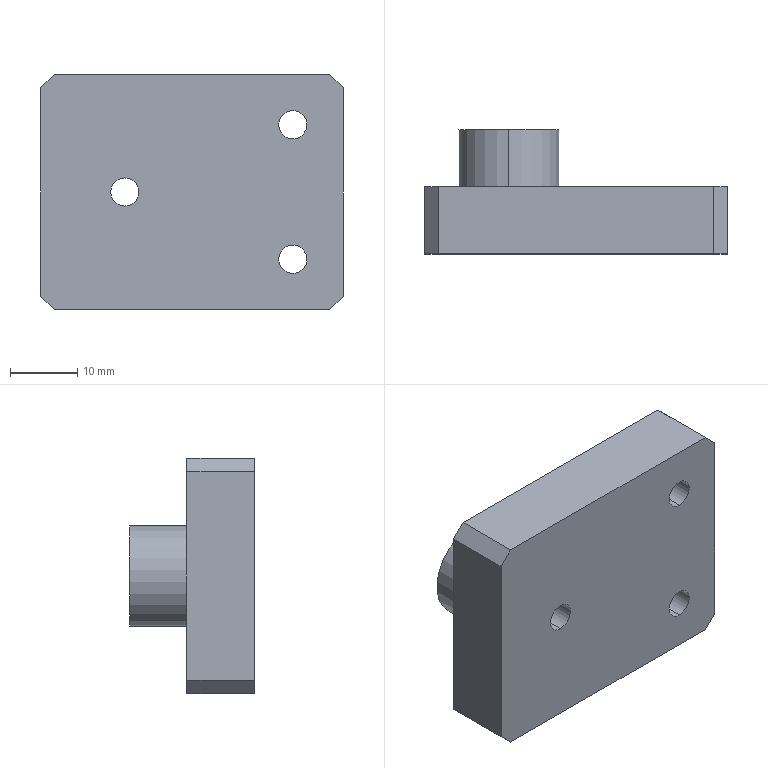Part | SolidWorks | features HoleWzd 2, ICE 2, Chamfer 1, Extrusion 1 | 1 solid | 19 faces | box 45 x 18.5 x 35 mm | volume 16639 mm3 | plane 11 | cylinder 8 | commonest cylinder face diameters 4.2 x6 15 x2
STEP:
#1=CARTESIAN_POINT('',(-10.,-5.,-2.1));
#2=VERTEX_POINT('',#1);
#3=CARTESIAN_POINT('',(-10.,-5.,2.1));
#4=VERTEX_POINT('',#3);
#5=CARTESIAN_POINT('',(-10.,-5.,0.));
#6=DIRECTION('',(0.,1.,0.));
#7=DIRECTION('',(0.,0.,1.));
#8=AXIS2_PLACEMENT_3D('',#5,#6,#7);
#9=CIRCLE('',#8,2.1);
#10=EDGE_CURVE('',#2,#4,#9,.T.);
#11=ORIENTED_EDGE('',*,*,#10,.F.);
#12=CARTESIAN_POINT('',(-10.,13.5,-2.1));
#13=VERTEX_POINT('',#12);
#14=CARTESIAN_POINT('',(-10.,13.5,-2.1));
#15=DIRECTION('',(0.,1.,0.));
#16=VECTOR('',#15,1000.);
#17=LINE('',#14,#16);
#18=EDGE_CURVE('',#2,#13,#17,.T.);
#19=ORIENTED_EDGE('',*,*,#18,.T.);
#20=CARTESIAN_POINT('',(-10.,13.5,2.1));
#21=VERTEX_POINT('',#20);
#22=CARTESIAN_POINT('',(-10.,13.5,0.));
#23=DIRECTION('',(0.,1.,0.));
#24=DIRECTION('',(0.,0.,1.));
#25=AXIS2_PLACEMENT_3D('',#22,#23,#24);
#26=CIRCLE('',#25,2.1);
#27=EDGE_CURVE('',#13,#21,#26,.T.);
#28=ORIENTED_EDGE('',*,*,#27,.T.);
#29=CARTESIAN_POINT('',(-10.,13.5,2.1));
#30=DIRECTION('',(0.,1.,0.));
#31=VECTOR('',#30,1000.);
#32=LINE('',#29,#31);
#33=EDGE_CURVE('',#4,#21,#32,.T.);
#34=ORIENTED_EDGE('',*,*,#33,.F.);
#35=EDGE_LOOP('',(#11,#19,#28,#34));
#36=FACE_OUTER_BOUND('',#35,.T.);
#37=CARTESIAN_POINT('',(-10.,13.5,0.));
#38=DIRECTION('',(0.,1.,0.));
#39=DIRECTION('',(0.,0.,1.));
#40=AXIS2_PLACEMENT_3D('',#37,#38,#39);
#41=CYLINDRICAL_SURFACE('',#40,2.1);
#42=ADVANCED_FACE('',(#36),#41,.F.);
#43=CARTESIAN_POINT('',(15.,-5.,7.9));
#44=VERTEX_POINT('',#43);
#45=CARTESIAN_POINT('',(15.,-5.,12.1));
#46=VERTEX_POINT('',#45);
#47=CARTESIAN_POINT('',(15.,-5.,10.));
#48=DIRECTION('',(0.,1.,0.));
#49=DIRECTION('',(0.,0.,1.));
#50=AXIS2_PLACEMENT_3D('',#47,#48,#49);
#51=CIRCLE('',#50,2.1);
#52=EDGE_CURVE('',#44,#46,#51,.T.);
#53=ORIENTED_EDGE('',*,*,#52,.F.);
#54=CARTESIAN_POINT('',(15.,5.,7.9));
#55=VERTEX_POINT('',#54);
#56=CARTESIAN_POINT('',(15.,5.,7.9));
#57=DIRECTION('',(0.,1.,0.));
#58=VECTOR('',#57,1000.);
#59=LINE('',#56,#58);
#60=EDGE_CURVE('',#44,#55,#59,.T.);
#61=ORIENTED_EDGE('',*,*,#60,.T.);
#62=CARTESIAN_POINT('',(15.,5.,12.1));
#63=VERTEX_POINT('',#62);
#64=CARTESIAN_POINT('',(15.,5.,10.));
#65=DIRECTION('',(0.,1.,0.));
#66=DIRECTION('',(0.,0.,1.));
#67=AXIS2_PLACEMENT_3D('',#64,#65,#66);
#68=CIRCLE('',#67,2.1);
#69=EDGE_CURVE('',#55,#63,#68,.T.);
#70=ORIENTED_EDGE('',*,*,#69,.T.);
#71=CARTESIAN_POINT('',(15.,5.,12.1));
#72=DIRECTION('',(0.,1.,0.));
#73=VECTOR('',#72,1000.);
#74=LINE('',#71,#73);
#75=EDGE_CURVE('',#46,#63,#74,.T.);
#76=ORIENTED_EDGE('',*,*,#75,.F.);
#77=EDGE_LOOP('',(#53,#61,#70,#76));
#78=FACE_OUTER_BOUND('',#77,.T.);
#79=CARTESIAN_POINT('',(15.,5.,10.));
#80=DIRECTION('',(0.,1.,0.));
#81=DIRECTION('',(0.,0.,1.));
#82=AXIS2_PLACEMENT_3D('',#79,#80,#81);
#83=CYLINDRICAL_SURFACE('',#82,2.1);
#84=ADVANCED_FACE('',(#78),#83,.F.);
#85=CARTESIAN_POINT('',(15.,-5.,-12.1));
#86=VERTEX_POINT('',#85);
#87=CARTESIAN_POINT('',(15.,-5.,-7.9));
#88=VERTEX_POINT('',#87);
#89=CARTESIAN_POINT('',(15.,-5.,-10.));
#90=DIRECTION('',(0.,1.,0.));
#91=DIRECTION('',(0.,0.,1.));
#92=AXIS2_PLACEMENT_3D('',#89,#90,#91);
#93=CIRCLE('',#92,2.1);
#94=EDGE_CURVE('',#86,#88,#93,.T.);
#95=ORIENTED_EDGE('',*,*,#94,.F.);
#96=CARTESIAN_POINT('',(15.,5.,-12.1));
#97=VERTEX_POINT('',#96);
#98=CARTESIAN_POINT('',(15.,5.,-12.1));
#99=DIRECTION('',(0.,1.,0.));
#100=VECTOR('',#99,1000.);
#101=LINE('',#98,#100);
#102=EDGE_CURVE('',#86,#97,#101,.T.);
#103=ORIENTED_EDGE('',*,*,#102,.T.);
#104=CARTESIAN_POINT('',(15.,5.,-7.9));
#105=VERTEX_POINT('',#104);
#106=CARTESIAN_POINT('',(15.,5.,-10.));
#107=DIRECTION('',(0.,1.,0.));
#108=DIRECTION('',(0.,0.,1.));
#109=AXIS2_PLACEMENT_3D('',#106,#107,#108);
#110=CIRCLE('',#109,2.1);
#111=EDGE_CURVE('',#97,#105,#110,.T.);
#112=ORIENTED_EDGE('',*,*,#111,.T.);
#113=CARTESIAN_POINT('',(15.,5.,-7.9));
#114=DIRECTION('',(0.,1.,0.));
#115=VECTOR('',#114,1000.);
#116=LINE('',#113,#115);
#117=EDGE_CURVE('',#88,#105,#116,.T.);
#118=ORIENTED_EDGE('',*,*,#117,.F.);
#119=EDGE_LOOP('',(#95,#103,#112,#118));
#120=FACE_OUTER_BOUND('',#119,.T.);
#121=CARTESIAN_POINT('',(15.,5.,-10.));
#122=DIRECTION('',(0.,1.,0.));
#123=DIRECTION('',(0.,0.,1.));
#124=AXIS2_PLACEMENT_3D('',#121,#122,#123);
#125=CYLINDRICAL_SURFACE('',#124,2.1);
#126=ADVANCED_FACE('',(#120),#125,.F.);
#127=CARTESIAN_POINT('',(-10.,13.5,7.5));
#128=VERTEX_POINT('',#127);
#129=CARTESIAN_POINT('',(-10.,13.5,-7.5));
#130=VERTEX_POINT('',#129);
#131=CARTESIAN_POINT('',(-10.,13.5,0.));
#132=DIRECTION('',(0.,1.,0.));
#133=DIRECTION('',(0.,0.,1.));
#134=AXIS2_PLACEMENT_3D('',#131,#132,#133);
#135=CIRCLE('',#134,7.5);
#136=EDGE_CURVE('',#128,#130,#135,.T.);
#137=ORIENTED_EDGE('',*,*,#136,.F.);
#138=CARTESIAN_POINT('',(-10.,5.,7.5));
#139=VERTEX_POINT('',#138);
#140=CARTESIAN_POINT('',(-10.,13.5,7.5));
#141=DIRECTION('',(0.,-1.,0.));
#142=VECTOR('',#141,1000.);
#143=LINE('',#140,#142);
#144=EDGE_CURVE('',#128,#139,#143,.T.);
#145=ORIENTED_EDGE('',*,*,#144,.T.);
#146=CARTESIAN_POINT('',(-10.,5.,-7.5));
#147=VERTEX_POINT('',#146);
#148=CARTESIAN_POINT('',(-10.,5.,0.));
#149=DIRECTION('',(0.,1.,0.));
#150=DIRECTION('',(0.,0.,-1.));
#151=AXIS2_PLACEMENT_3D('',#148,#149,#150);
#152=CIRCLE('',#151,7.5);
#153=EDGE_CURVE('',#139,#147,#152,.T.);
#154=ORIENTED_EDGE('',*,*,#153,.T.);
#155=CARTESIAN_POINT('',(-10.,13.5,-7.5));
#156=DIRECTION('',(0.,-1.,0.));
#157=VECTOR('',#156,1000.);
#158=LINE('',#155,#157);
#159=EDGE_CURVE('',#130,#147,#158,.T.);
#160=ORIENTED_EDGE('',*,*,#159,.F.);
#161=EDGE_LOOP('',(#137,#145,#154,#160));
#162=FACE_OUTER_BOUND('',#161,.T.);
#163=CARTESIAN_POINT('',(-10.,13.5,0.));
#164=DIRECTION('',(0.,-1.,0.));
#165=DIRECTION('',(0.,0.,-1.));
#166=AXIS2_PLACEMENT_3D('',#163,#164,#165);
#167=CYLINDRICAL_SURFACE('',#166,7.5);
#168=ADVANCED_FACE('',(#162),#167,.T.);
#169=CARTESIAN_POINT('',(-10.,-5.,0.));
#170=DIRECTION('',(0.,1.,0.));
#171=DIRECTION('',(0.,0.,1.));
#172=AXIS2_PLACEMENT_3D('',#169,#170,#171);
#173=CIRCLE('',#172,2.1);
#174=EDGE_CURVE('',#4,#2,#173,.T.);
#175=ORIENTED_EDGE('',*,*,#174,.T.);
#176=ORIENTED_EDGE('',*,*,#10,.T.);
#177=EDGE_LOOP('',(#175,#176));
#178=FACE_BOUND('',#177,.T.);
#179=CARTESIAN_POINT('',(22.5,-5.,15.5));
#180=VERTEX_POINT('',#179);
#181=CARTESIAN_POINT('',(22.5,-5.,-15.5));
#182=VERTEX_POINT('',#181);
#183=CARTESIAN_POINT('',(22.5,-5.,17.5));
#184=DIRECTION('',(0.,0.,-1.));
#185=VECTOR('',#184,1000.);
#186=LINE('',#183,#185);
#187=EDGE_CURVE('',#180,#182,#186,.T.);
#188=ORIENTED_EDGE('',*,*,#187,.F.);
#189=CARTESIAN_POINT('',(20.5,-5.,17.5));
#190=VERTEX_POINT('',#189);
#191=CARTESIAN_POINT('',(19.,-5.,19.));
#192=DIRECTION('',(-0.7071,0.,0.7071));
#193=VECTOR('',#192,1000.);
#194=LINE('',#191,#193);
#195=EDGE_CURVE('',#180,#190,#194,.T.);
#196=ORIENTED_EDGE('',*,*,#195,.T.);
#197=CARTESIAN_POINT('',(-20.5,-5.,17.5));
#198=VERTEX_POINT('',#197);
#199=CARTESIAN_POINT('',(-22.5,-5.,17.5));
#200=DIRECTION('',(1.,0.,0.));
#201=VECTOR('',#200,1000.);
#202=LINE('',#199,#201);
#203=EDGE_CURVE('',#198,#190,#202,.T.);
#204=ORIENTED_EDGE('',*,*,#203,.F.);
#205=CARTESIAN_POINT('',(-22.5,-5.,15.5));
#206=VERTEX_POINT('',#205);
#207=CARTESIAN_POINT('',(-19.,-5.,19.));
#208=DIRECTION('',(-0.7071,0.,-0.7071));
#209=VECTOR('',#208,1000.);
#210=LINE('',#207,#209);
#211=EDGE_CURVE('',#198,#206,#210,.T.);
#212=ORIENTED_EDGE('',*,*,#211,.T.);
#213=CARTESIAN_POINT('',(-22.5,-5.,-15.5));
#214=VERTEX_POINT('',#213);
#215=CARTESIAN_POINT('',(-22.5,-5.,17.5));
#216=DIRECTION('',(0.,0.,1.));
#217=VECTOR('',#216,1000.);
#218=LINE('',#215,#217);
#219=EDGE_CURVE('',#214,#206,#218,.T.);
#220=ORIENTED_EDGE('',*,*,#219,.F.);
#221=CARTESIAN_POINT('',(-20.5,-5.,-17.5));
#222=VERTEX_POINT('',#221);
#223=CARTESIAN_POINT('',(-19.,-5.,-19.));
#224=DIRECTION('',(0.7071,0.,-0.7071));
#225=VECTOR('',#224,1000.);
#226=LINE('',#223,#225);
#227=EDGE_CURVE('',#214,#222,#226,.T.);
#228=ORIENTED_EDGE('',*,*,#227,.T.);
#229=CARTESIAN_POINT('',(20.5,-5.,-17.5));
#230=VERTEX_POINT('',#229);
#231=CARTESIAN_POINT('',(-22.5,-5.,-17.5));
#232=DIRECTION('',(-1.,0.,0.));
#233=VECTOR('',#232,1000.);
#234=LINE('',#231,#233);
#235=EDGE_CURVE('',#230,#222,#234,.T.);
#236=ORIENTED_EDGE('',*,*,#235,.F.);
#237=CARTESIAN_POINT('',(19.,-5.,-19.));
#238=DIRECTION('',(0.7071,0.,0.7071));
#239=VECTOR('',#238,1000.);
#240=LINE('',#237,#239);
#241=EDGE_CURVE('',#230,#182,#240,.T.);
#242=ORIENTED_EDGE('',*,*,#241,.T.);
#243=EDGE_LOOP('',(#188,#196,#204,#212,#220,#228,#236,#242));
#244=FACE_OUTER_BOUND('',#243,.T.);
#245=CARTESIAN_POINT('',(15.,-5.,-10.));
#246=DIRECTION('',(0.,1.,0.));
#247=DIRECTION('',(0.,0.,1.));
#248=AXIS2_PLACEMENT_3D('',#245,#246,#247);
#249=CIRCLE('',#248,2.1);
#250=EDGE_CURVE('',#88,#86,#249,.T.);
#251=ORIENTED_EDGE('',*,*,#250,.T.);
#252=ORIENTED_EDGE('',*,*,#94,.T.);
#253=EDGE_LOOP('',(#251,#252));
#254=FACE_BOUND('',#253,.T.);
#255=CARTESIAN_POINT('',(15.,-5.,10.));
#256=DIRECTION('',(0.,1.,0.));
#257=DIRECTION('',(0.,0.,1.));
#258=AXIS2_PLACEMENT_3D('',#255,#256,#257);
#259=CIRCLE('',#258,2.1);
#260=EDGE_CURVE('',#46,#44,#259,.T.);
#261=ORIENTED_EDGE('',*,*,#260,.T.);
#262=ORIENTED_EDGE('',*,*,#52,.T.);
#263=EDGE_LOOP('',(#261,#262));
#264=FACE_BOUND('',#263,.T.);
#265=CARTESIAN_POINT('',(0.,-5.,0.));
#266=DIRECTION('',(0.,-1.,0.));
#267=DIRECTION('',(0.,0.,-1.));
#268=AXIS2_PLACEMENT_3D('',#265,#266,#267);
#269=PLANE('',#268);
#270=ADVANCED_FACE('',(#178,#244,#254,#264),#269,.T.);
#271=CARTESIAN_POINT('',(22.5,5.,15.5));
#272=VERTEX_POINT('',#271);
#273=CARTESIAN_POINT('',(22.5,5.,-15.5));
#274=VERTEX_POINT('',#273);
#275=CARTESIAN_POINT('',(22.5,5.,17.5));
#276=DIRECTION('',(0.,0.,-1.));
#277=VECTOR('',#276,1000.);
#278=LINE('',#275,#277);
#279=EDGE_CURVE('',#272,#274,#278,.T.);
#280=ORIENTED_EDGE('',*,*,#279,.F.);
#281=CARTESIAN_POINT('',(22.5,5.,15.5));
#282=DIRECTION('',(0.,-1.,0.));
#283=VECTOR('',#282,1000.);
#284=LINE('',#281,#283);
#285=EDGE_CURVE('',#272,#180,#284,.T.);
#286=ORIENTED_EDGE('',*,*,#285,.T.);
#287=ORIENTED_EDGE('',*,*,#187,.T.);
#288=CARTESIAN_POINT('',(22.5,5.,-15.5));
#289=DIRECTION('',(0.,1.,0.));
#290=VECTOR('',#289,1000.);
#291=LINE('',#288,#290);
#292=EDGE_CURVE('',#182,#274,#291,.T.);
#293=ORIENTED_EDGE('',*,*,#292,.T.);
#294=EDGE_LOOP('',(#280,#286,#287,#293));
#295=FACE_OUTER_BOUND('',#294,.T.);
#296=CARTESIAN_POINT('',(22.5,5.,17.5));
#297=DIRECTION('',(-1.,0.,0.));
#298=DIRECTION('',(0.,0.,1.));
#299=AXIS2_PLACEMENT_3D('',#296,#297,#298);
#300=PLANE('',#299);
#301=ADVANCED_FACE('',(#295),#300,.F.);
#302=CARTESIAN_POINT('',(20.5,5.,-17.5));
#303=VERTEX_POINT('',#302);
#304=CARTESIAN_POINT('',(-20.5,5.,-17.5));
#305=VERTEX_POINT('',#304);
#306=CARTESIAN_POINT('',(-22.5,5.,-17.5));
#307=DIRECTION('',(-1.,0.,0.));
#308=VECTOR('',#307,1000.);
#309=LINE('',#306,#308);
#310=EDGE_CURVE('',#303,#305,#309,.T.);
#311=ORIENTED_EDGE('',*,*,#310,.F.);
#312=CARTESIAN_POINT('',(20.5,5.,-17.5));
#313=DIRECTION('',(0.,-1.,0.));
#314=VECTOR('',#313,1000.);
#315=LINE('',#312,#314);
#316=EDGE_CURVE('',#303,#230,#315,.T.);
#317=ORIENTED_EDGE('',*,*,#316,.T.);
#318=ORIENTED_EDGE('',*,*,#235,.T.);
#319=CARTESIAN_POINT('',(-20.5,5.,-17.5));
#320=DIRECTION('',(0.,1.,0.));
#321=VECTOR('',#320,1000.);
#322=LINE('',#319,#321);
#323=EDGE_CURVE('',#222,#305,#322,.T.);
#324=ORIENTED_EDGE('',*,*,#323,.T.);
#325=EDGE_LOOP('',(#311,#317,#318,#324));
#326=FACE_OUTER_BOUND('',#325,.T.);
#327=CARTESIAN_POINT('',(-22.5,5.,-17.5));
#328=DIRECTION('',(0.,0.,1.));
#329=DIRECTION('',(1.,0.,0.));
#330=AXIS2_PLACEMENT_3D('',#327,#328,#329);
#331=PLANE('',#330);
#332=ADVANCED_FACE('',(#326),#331,.F.);
#333=ORIENTED_EDGE('',*,*,#219,.T.);
#334=CARTESIAN_POINT('',(-22.5,5.,15.5));
#335=VERTEX_POINT('',#334);
#336=CARTESIAN_POINT('',(-22.5,5.,15.5));
#337=DIRECTION('',(0.,1.,0.));
#338=VECTOR('',#337,1000.);
#339=LINE('',#336,#338);
#340=EDGE_CURVE('',#206,#335,#339,.T.);
#341=ORIENTED_EDGE('',*,*,#340,.T.);
#342=CARTESIAN_POINT('',(-22.5,5.,-15.5));
#343=VERTEX_POINT('',#342);
#344=CARTESIAN_POINT('',(-22.5,5.,17.5));
#345=DIRECTION('',(0.,0.,1.));
#346=VECTOR('',#345,1000.);
#347=LINE('',#344,#346);
#348=EDGE_CURVE('',#343,#335,#347,.T.);
#349=ORIENTED_EDGE('',*,*,#348,.F.);
#350=CARTESIAN_POINT('',(-22.5,5.,-15.5));
#351=DIRECTION('',(0.,-1.,0.));
#352=VECTOR('',#351,1000.);
#353=LINE('',#350,#352);
#354=EDGE_CURVE('',#343,#214,#353,.T.);
#355=ORIENTED_EDGE('',*,*,#354,.T.);
#356=EDGE_LOOP('',(#333,#341,#349,#355));
#357=FACE_OUTER_BOUND('',#356,.T.);
#358=CARTESIAN_POINT('',(-22.5,5.,17.5));
#359=DIRECTION('',(1.,0.,0.));
#360=DIRECTION('',(0.,0.,-1.));
#361=AXIS2_PLACEMENT_3D('',#358,#359,#360);
#362=PLANE('',#361);
#363=ADVANCED_FACE('',(#357),#362,.F.);
#364=ORIENTED_EDGE('',*,*,#203,.T.);
#365=CARTESIAN_POINT('',(20.5,5.,17.5));
#366=VERTEX_POINT('',#365);
#367=CARTESIAN_POINT('',(20.5,5.,17.5));
#368=DIRECTION('',(0.,1.,0.));
#369=VECTOR('',#368,1000.);
#370=LINE('',#367,#369);
#371=EDGE_CURVE('',#190,#366,#370,.T.);
#372=ORIENTED_EDGE('',*,*,#371,.T.);
#373=CARTESIAN_POINT('',(-20.5,5.,17.5));
#374=VERTEX_POINT('',#373);
#375=CARTESIAN_POINT('',(-22.5,5.,17.5));
#376=DIRECTION('',(1.,0.,0.));
#377=VECTOR('',#376,1000.);
#378=LINE('',#375,#377);
#379=EDGE_CURVE('',#374,#366,#378,.T.);
#380=ORIENTED_EDGE('',*,*,#379,.F.);
#381=CARTESIAN_POINT('',(-20.5,5.,17.5));
#382=DIRECTION('',(0.,-1.,0.));
#383=VECTOR('',#382,1000.);
#384=LINE('',#381,#383);
#385=EDGE_CURVE('',#374,#198,#384,.T.);
#386=ORIENTED_EDGE('',*,*,#385,.T.);
#387=EDGE_LOOP('',(#364,#372,#380,#386));
#388=FACE_OUTER_BOUND('',#387,.T.);
#389=CARTESIAN_POINT('',(-22.5,5.,17.5));
#390=DIRECTION('',(0.,0.,-1.));
#391=DIRECTION('',(-1.,0.,0.));
#392=AXIS2_PLACEMENT_3D('',#389,#390,#391);
#393=PLANE('',#392);
#394=ADVANCED_FACE('',(#388),#393,.F.);
#395=CARTESIAN_POINT('',(15.,5.,10.));
#396=DIRECTION('',(0.,1.,0.));
#397=DIRECTION('',(0.,0.,1.));
#398=AXIS2_PLACEMENT_3D('',#395,#396,#397);
#399=CIRCLE('',#398,2.1);
#400=EDGE_CURVE('',#63,#55,#399,.T.);
#401=ORIENTED_EDGE('',*,*,#400,.F.);
#402=ORIENTED_EDGE('',*,*,#69,.F.);
#403=EDGE_LOOP('',(#401,#402));
#404=FACE_BOUND('',#403,.T.);
#405=CARTESIAN_POINT('',(15.,5.,-10.));
#406=DIRECTION('',(0.,1.,0.));
#407=DIRECTION('',(0.,0.,1.));
#408=AXIS2_PLACEMENT_3D('',#405,#406,#407);
#409=CIRCLE('',#408,2.1);
#410=EDGE_CURVE('',#105,#97,#409,.T.);
#411=ORIENTED_EDGE('',*,*,#410,.F.);
#412=ORIENTED_EDGE('',*,*,#111,.F.);
#413=EDGE_LOOP('',(#411,#412));
#414=FACE_BOUND('',#413,.T.);
#415=CARTESIAN_POINT('',(-10.,5.,0.));
#416=DIRECTION('',(0.,1.,0.));
#417=DIRECTION('',(0.,0.,-1.));
#418=AXIS2_PLACEMENT_3D('',#415,#416,#417);
#419=CIRCLE('',#418,7.5);
#420=EDGE_CURVE('',#147,#139,#419,.T.);
#421=ORIENTED_EDGE('',*,*,#420,.F.);
#422=ORIENTED_EDGE('',*,*,#153,.F.);
#423=EDGE_LOOP('',(#421,#422));
#424=FACE_BOUND('',#423,.T.);
#425=ORIENTED_EDGE('',*,*,#379,.T.);
#426=CARTESIAN_POINT('',(22.5,5.,15.5));
#427=DIRECTION('',(0.7071,0.,-0.7071));
#428=VECTOR('',#427,1000.);
#429=LINE('',#426,#428);
#430=EDGE_CURVE('',#366,#272,#429,.T.);
#431=ORIENTED_EDGE('',*,*,#430,.T.);
#432=ORIENTED_EDGE('',*,*,#279,.T.);
#433=CARTESIAN_POINT('',(20.5,5.,-17.5));
#434=DIRECTION('',(-0.7071,0.,-0.7071));
#435=VECTOR('',#434,1000.);
#436=LINE('',#433,#435);
#437=EDGE_CURVE('',#274,#303,#436,.T.);
#438=ORIENTED_EDGE('',*,*,#437,.T.);
#439=ORIENTED_EDGE('',*,*,#310,.T.);
#440=CARTESIAN_POINT('',(-22.5,5.,-15.5));
#441=DIRECTION('',(-0.7071,0.,0.7071));
#442=VECTOR('',#441,1000.);
#443=LINE('',#440,#442);
#444=EDGE_CURVE('',#305,#343,#443,.T.);
#445=ORIENTED_EDGE('',*,*,#444,.T.);
#446=ORIENTED_EDGE('',*,*,#348,.T.);
#447=CARTESIAN_POINT('',(-20.5,5.,17.5));
#448=DIRECTION('',(0.7071,0.,0.7071));
#449=VECTOR('',#448,1000.);
#450=LINE('',#447,#449);
#451=EDGE_CURVE('',#335,#374,#450,.T.);
#452=ORIENTED_EDGE('',*,*,#451,.T.);
#453=EDGE_LOOP('',(#425,#431,#432,#438,#439,#445,#446,#452));
#454=FACE_OUTER_BOUND('',#453,.T.);
#455=CARTESIAN_POINT('',(0.,5.,0.));
#456=DIRECTION('',(0.,-1.,0.));
#457=DIRECTION('',(0.,0.,-1.));
#458=AXIS2_PLACEMENT_3D('',#455,#456,#457);
#459=PLANE('',#458);
#460=ADVANCED_FACE('',(#404,#414,#424,#454),#459,.F.);
#461=ORIENTED_EDGE('',*,*,#430,.F.);
#462=ORIENTED_EDGE('',*,*,#371,.F.);
#463=ORIENTED_EDGE('',*,*,#195,.F.);
#464=ORIENTED_EDGE('',*,*,#285,.F.);
#465=EDGE_LOOP('',(#461,#462,#463,#464));
#466=FACE_OUTER_BOUND('',#465,.T.);
#467=CARTESIAN_POINT('',(22.5,5.,15.5));
#468=DIRECTION('',(-0.7071,0.,-0.7071));
#469=DIRECTION('',(0.,-1.,0.));
#470=AXIS2_PLACEMENT_3D('',#467,#468,#469);
#471=PLANE('',#470);
#472=ADVANCED_FACE('',(#466),#471,.F.);
#473=ORIENTED_EDGE('',*,*,#437,.F.);
#474=ORIENTED_EDGE('',*,*,#292,.F.);
#475=ORIENTED_EDGE('',*,*,#241,.F.);
#476=ORIENTED_EDGE('',*,*,#316,.F.);
#477=EDGE_LOOP('',(#473,#474,#475,#476));
#478=FACE_OUTER_BOUND('',#477,.T.);
#479=CARTESIAN_POINT('',(20.5,5.,-17.5));
#480=DIRECTION('',(-0.7071,0.,0.7071));
#481=DIRECTION('',(0.,-1.,0.));
#482=AXIS2_PLACEMENT_3D('',#479,#480,#481);
#483=PLANE('',#482);
#484=ADVANCED_FACE('',(#478),#483,.F.);
#485=ORIENTED_EDGE('',*,*,#451,.F.);
#486=ORIENTED_EDGE('',*,*,#340,.F.);
#487=ORIENTED_EDGE('',*,*,#211,.F.);
#488=ORIENTED_EDGE('',*,*,#385,.F.);
#489=EDGE_LOOP('',(#485,#486,#487,#488));
#490=FACE_OUTER_BOUND('',#489,.T.);
#491=CARTESIAN_POINT('',(-20.5,5.,17.5));
#492=DIRECTION('',(0.7071,0.,-0.7071));
#493=DIRECTION('',(0.,-1.,0.));
#494=AXIS2_PLACEMENT_3D('',#491,#492,#493);
#495=PLANE('',#494);
#496=ADVANCED_FACE('',(#490),#495,.F.);
#497=ORIENTED_EDGE('',*,*,#444,.F.);
#498=ORIENTED_EDGE('',*,*,#323,.F.);
#499=ORIENTED_EDGE('',*,*,#227,.F.);
#500=ORIENTED_EDGE('',*,*,#354,.F.);
#501=EDGE_LOOP('',(#497,#498,#499,#500));
#502=FACE_OUTER_BOUND('',#501,.T.);
#503=CARTESIAN_POINT('',(-22.5,5.,-15.5));
#504=DIRECTION('',(0.7071,0.,0.7071));
#505=DIRECTION('',(0.,-1.,0.));
#506=AXIS2_PLACEMENT_3D('',#503,#504,#505);
#507=PLANE('',#506);
#508=ADVANCED_FACE('',(#502),#507,.F.);
#509=ORIENTED_EDGE('',*,*,#144,.F.);
#510=CARTESIAN_POINT('',(-10.,13.5,0.));
#511=DIRECTION('',(0.,1.,0.));
#512=DIRECTION('',(0.,0.,1.));
#513=AXIS2_PLACEMENT_3D('',#510,#511,#512);
#514=CIRCLE('',#513,7.5);
#515=EDGE_CURVE('',#130,#128,#514,.T.);
#516=ORIENTED_EDGE('',*,*,#515,.F.);
#517=ORIENTED_EDGE('',*,*,#159,.T.);
#518=ORIENTED_EDGE('',*,*,#420,.T.);
#519=EDGE_LOOP('',(#509,#516,#517,#518));
#520=FACE_OUTER_BOUND('',#519,.T.);
#521=CARTESIAN_POINT('',(-10.,13.5,0.));
#522=DIRECTION('',(0.,-1.,0.));
#523=DIRECTION('',(0.,0.,-1.));
#524=AXIS2_PLACEMENT_3D('',#521,#522,#523);
#525=CYLINDRICAL_SURFACE('',#524,7.5);
#526=ADVANCED_FACE('',(#520),#525,.T.);
#527=CARTESIAN_POINT('',(-10.,13.5,0.));
#528=DIRECTION('',(0.,1.,0.));
#529=DIRECTION('',(0.,0.,1.));
#530=AXIS2_PLACEMENT_3D('',#527,#528,#529);
#531=CIRCLE('',#530,2.1);
#532=EDGE_CURVE('',#21,#13,#531,.T.);
#533=ORIENTED_EDGE('',*,*,#532,.F.);
#534=ORIENTED_EDGE('',*,*,#27,.F.);
#535=EDGE_LOOP('',(#533,#534));
#536=FACE_BOUND('',#535,.T.);
#537=ORIENTED_EDGE('',*,*,#515,.T.);
#538=ORIENTED_EDGE('',*,*,#136,.T.);
#539=EDGE_LOOP('',(#537,#538));
#540=FACE_OUTER_BOUND('',#539,.T.);
#541=CARTESIAN_POINT('',(-10.,13.5,0.));
#542=DIRECTION('',(0.,1.,0.));
#543=DIRECTION('',(0.,0.,1.));
#544=AXIS2_PLACEMENT_3D('',#541,#542,#543);
#545=PLANE('',#544);
#546=ADVANCED_FACE('',(#536,#540),#545,.T.);
#547=ORIENTED_EDGE('',*,*,#102,.F.);
#548=ORIENTED_EDGE('',*,*,#250,.F.);
#549=ORIENTED_EDGE('',*,*,#117,.T.);
#550=ORIENTED_EDGE('',*,*,#410,.T.);
#551=EDGE_LOOP('',(#547,#548,#549,#550));
#552=FACE_OUTER_BOUND('',#551,.T.);
#553=CARTESIAN_POINT('',(15.,5.,-10.));
#554=DIRECTION('',(0.,1.,0.));
#555=DIRECTION('',(0.,0.,1.));
#556=AXIS2_PLACEMENT_3D('',#553,#554,#555);
#557=CYLINDRICAL_SURFACE('',#556,2.1);
#558=ADVANCED_FACE('',(#552),#557,.F.);
#559=ORIENTED_EDGE('',*,*,#60,.F.);
#560=ORIENTED_EDGE('',*,*,#260,.F.);
#561=ORIENTED_EDGE('',*,*,#75,.T.);
#562=ORIENTED_EDGE('',*,*,#400,.T.);
#563=EDGE_LOOP('',(#559,#560,#561,#562));
#564=FACE_OUTER_BOUND('',#563,.T.);
#565=CARTESIAN_POINT('',(15.,5.,10.));
#566=DIRECTION('',(0.,1.,0.));
#567=DIRECTION('',(0.,0.,1.));
#568=AXIS2_PLACEMENT_3D('',#565,#566,#567);
#569=CYLINDRICAL_SURFACE('',#568,2.1);
#570=ADVANCED_FACE('',(#564),#569,.F.);
#571=ORIENTED_EDGE('',*,*,#18,.F.);
#572=ORIENTED_EDGE('',*,*,#174,.F.);
#573=ORIENTED_EDGE('',*,*,#33,.T.);
#574=ORIENTED_EDGE('',*,*,#532,.T.);
#575=EDGE_LOOP('',(#571,#572,#573,#574));
#576=FACE_OUTER_BOUND('',#575,.T.);
#577=CARTESIAN_POINT('',(-10.,13.5,0.));
#578=DIRECTION('',(0.,1.,0.));
#579=DIRECTION('',(0.,0.,1.));
#580=AXIS2_PLACEMENT_3D('',#577,#578,#579);
#581=CYLINDRICAL_SURFACE('',#580,2.1);
#582=ADVANCED_FACE('',(#576),#581,.F.);
#583=CLOSED_SHELL('',(#42,#84,#126,#168,#270,#301,#332,#363,#394,#460,#472,#484,#496,#508,#526,#546,#558,#570,#582));
#584=MANIFOLD_SOLID_BREP('',#583);
#585=CARTESIAN_POINT('',(0.,0.,0.));
#586=DIRECTION('',(0.,0.,1.));
#587=DIRECTION('',(1.,0.,0.));
#588=AXIS2_PLACEMENT_3D('',#585,#586,#587);
#589=(LENGTH_UNIT()NAMED_UNIT(*)SI_UNIT(.MILLI.,.METRE.));
#590=UNCERTAINTY_MEASURE_WITH_UNIT(LENGTH_MEASURE(0.00001),#589,'','');
#591=(NAMED_UNIT(*)PLANE_ANGLE_UNIT()SI_UNIT($,.RADIAN.));
#592=(NAMED_UNIT(*)SI_UNIT($,.STERADIAN.)SOLID_ANGLE_UNIT());
#593=(GEOMETRIC_REPRESENTATION_CONTEXT(3)GLOBAL_UNCERTAINTY_ASSIGNED_CONTEXT((#590))GLOBAL_UNIT_ASSIGNED_CONTEXT((#589,#591,#592))REPRESENTATION_CONTEXT('',''));
#594=ADVANCED_BREP_SHAPE_REPRESENTATION('',(#584,#588),#593);